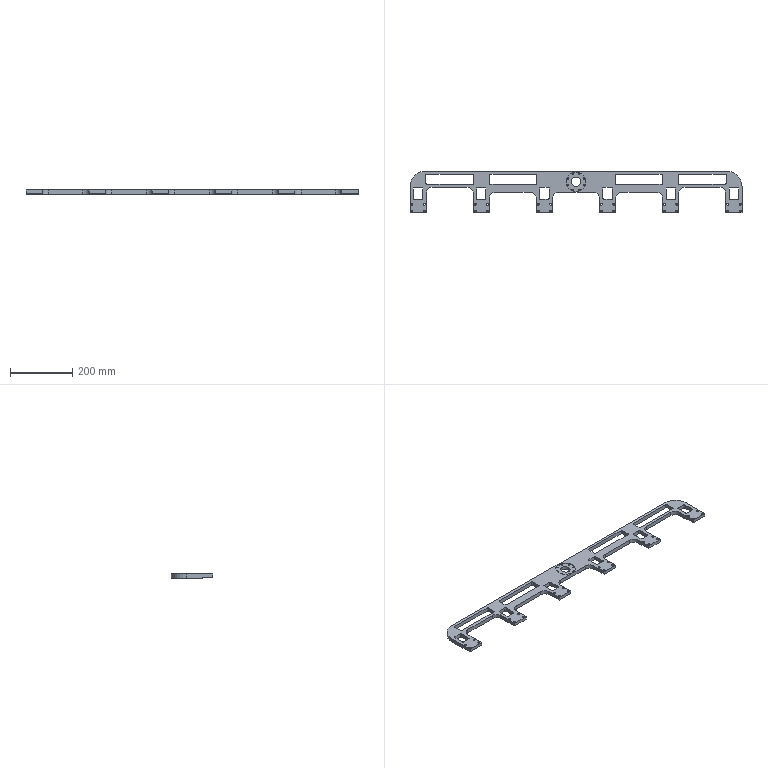NC program | NX | posted with a generic post | part box 1068 x 134 x 13 mm
Lines 1 to 125 of 9724:
N10 G17 G21 G94 G90
(FLOOR_WALL_COPY , TOOL : D63)
N12 T01 M6
N14 G54
N16 G17 G0 G90 X-572.5 Y70.997 S6500 M3
N18 G43 Z30. H1
N20 Z4.
N22 G94 G1 Z1. F1500.
N24 X-569.5
N26 X127.6
N28 Y41.798
N30 X-569.5
N32 Y12.599
N34 X127.6
N36 Y-16.601
N38 X-569.5
N40 Y-45.8
N42 X127.6
N44 Y-74.999
N46 X-569.5
N48 X-572.5
N50 Z4.
N52 G0 Z30.
N54 Y70.997
N56 Z3.
N58 G1 Z0.
N60 X-569.5
N62 X127.6
N64 Y41.798
N66 X-569.5
N68 Y12.599
N70 X127.6
N72 Y-16.601
N74 X-569.5
N76 Y-45.8
N78 X127.6
N80 Y-74.999
N82 X-569.5
N84 X-572.5
N86 Z3.
N88 G0 Z30.
N90 M5
(DRILLING_COPY_1 , TOOL : D6A45)
N92 T07 M6
N94 G54
N96 G17 G0 G90 X-528. Y-39.2 S5000 M3
N98 G43 Z30. H7
N100 G94 G81 G98 Z-1. F250. R3.
N102 Y-61.2
N104 X-488.
N106 Y-39.2
N108 X-324.8
N110 Y-61.2
N112 X-284.8
N114 Y-39.2
N116 X-121.6
N118 Y-61.2
N120 X-81.6
N122 Y-39.2
N124 X-25.869 Y22.285
N126 X-10.715 Y7.131
N128 X10.715
N130 X0. Y33.
N132 X-25.869 Y43.715
N134 X-10.715 Y58.869
N136 X10.715
N138 X25.869 Y43.715
N140 Y22.285
N142 X81.6 Y-39.2
N144 Y-61.2
N146 X121.6
N148 Y-39.2
N150 G80
N152 G0 X121.6 Y-39.2 Z30.
N154 M5
(DRILLING_COPY_COPY_1 , TOOL : 4.5ZT)
N156 T14 M6
N158 G54
N160 G17 G0 G90 X-25.869 Y22.285 S2000 M3
N162 G43 Z30. H14
N164 G94 G83 G98 Z-15.352 F250. Q2. R3.
N166 X-10.715 Y7.131
N168 X10.715
N170 X25.869 Y22.285
N172 Y43.715
N174 X10.715 Y58.869
N176 X-10.715
N178 X-25.869 Y43.715
N180 G80
N182 G0 X-25.869 Y43.715 Z30.
N184 M5
(DRILLING_COPY_COPY_COPY , TOOL : 6.5ZT)
N186 T15 M6
N188 G54
N190 G17 G0 G90 X-528. Y-61.2 S2000 M3
N192 G43 Z30. H15
N194 G94 G83 G98 Z-15.953 F250. Q2. R3.
N196 Y-39.2
N198 X-488.
N200 Y-61.2
N202 X-324.8
N204 Y-39.2
N206 X-284.8
N208 Y-61.2
N210 X-121.6
N212 Y-39.2
N214 X-81.6
N216 Y-61.2
N218 X81.6
N220 Y-39.2
N222 X121.6
N224 Y-61.2
N226 G80
N228 G0 X121.6 Y-61.2 Z30.
N230 M5